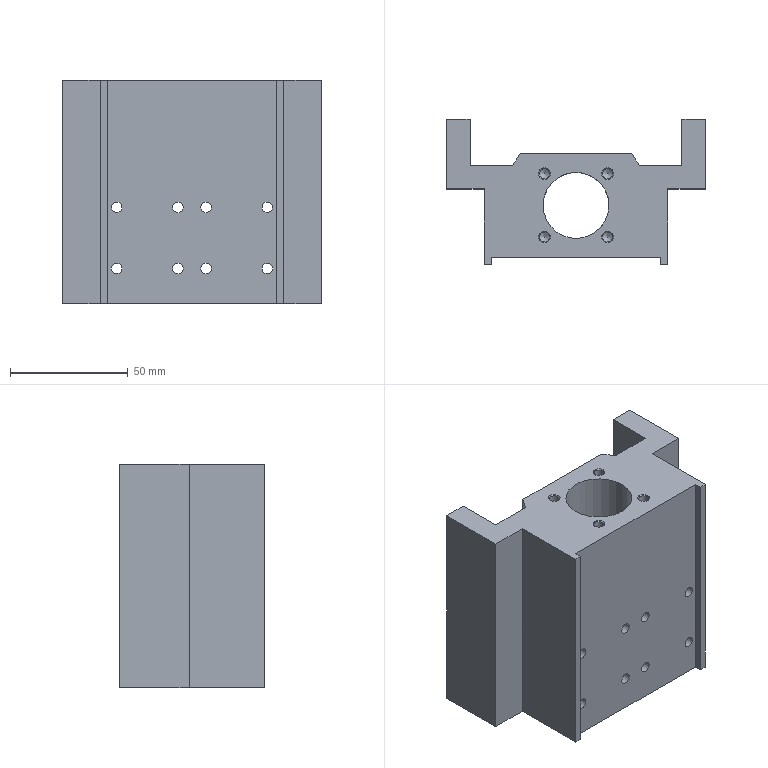Part | NX | 1 solid | 94 faces | box 110 x 61.5 x 95 mm | volume 250471 mm3 | plane 35 | cylinder 31 | cone 28 | commonest cylinder face diameters 4.2 x12 4.5 x8 7.5 x8 5 x2 28 x1